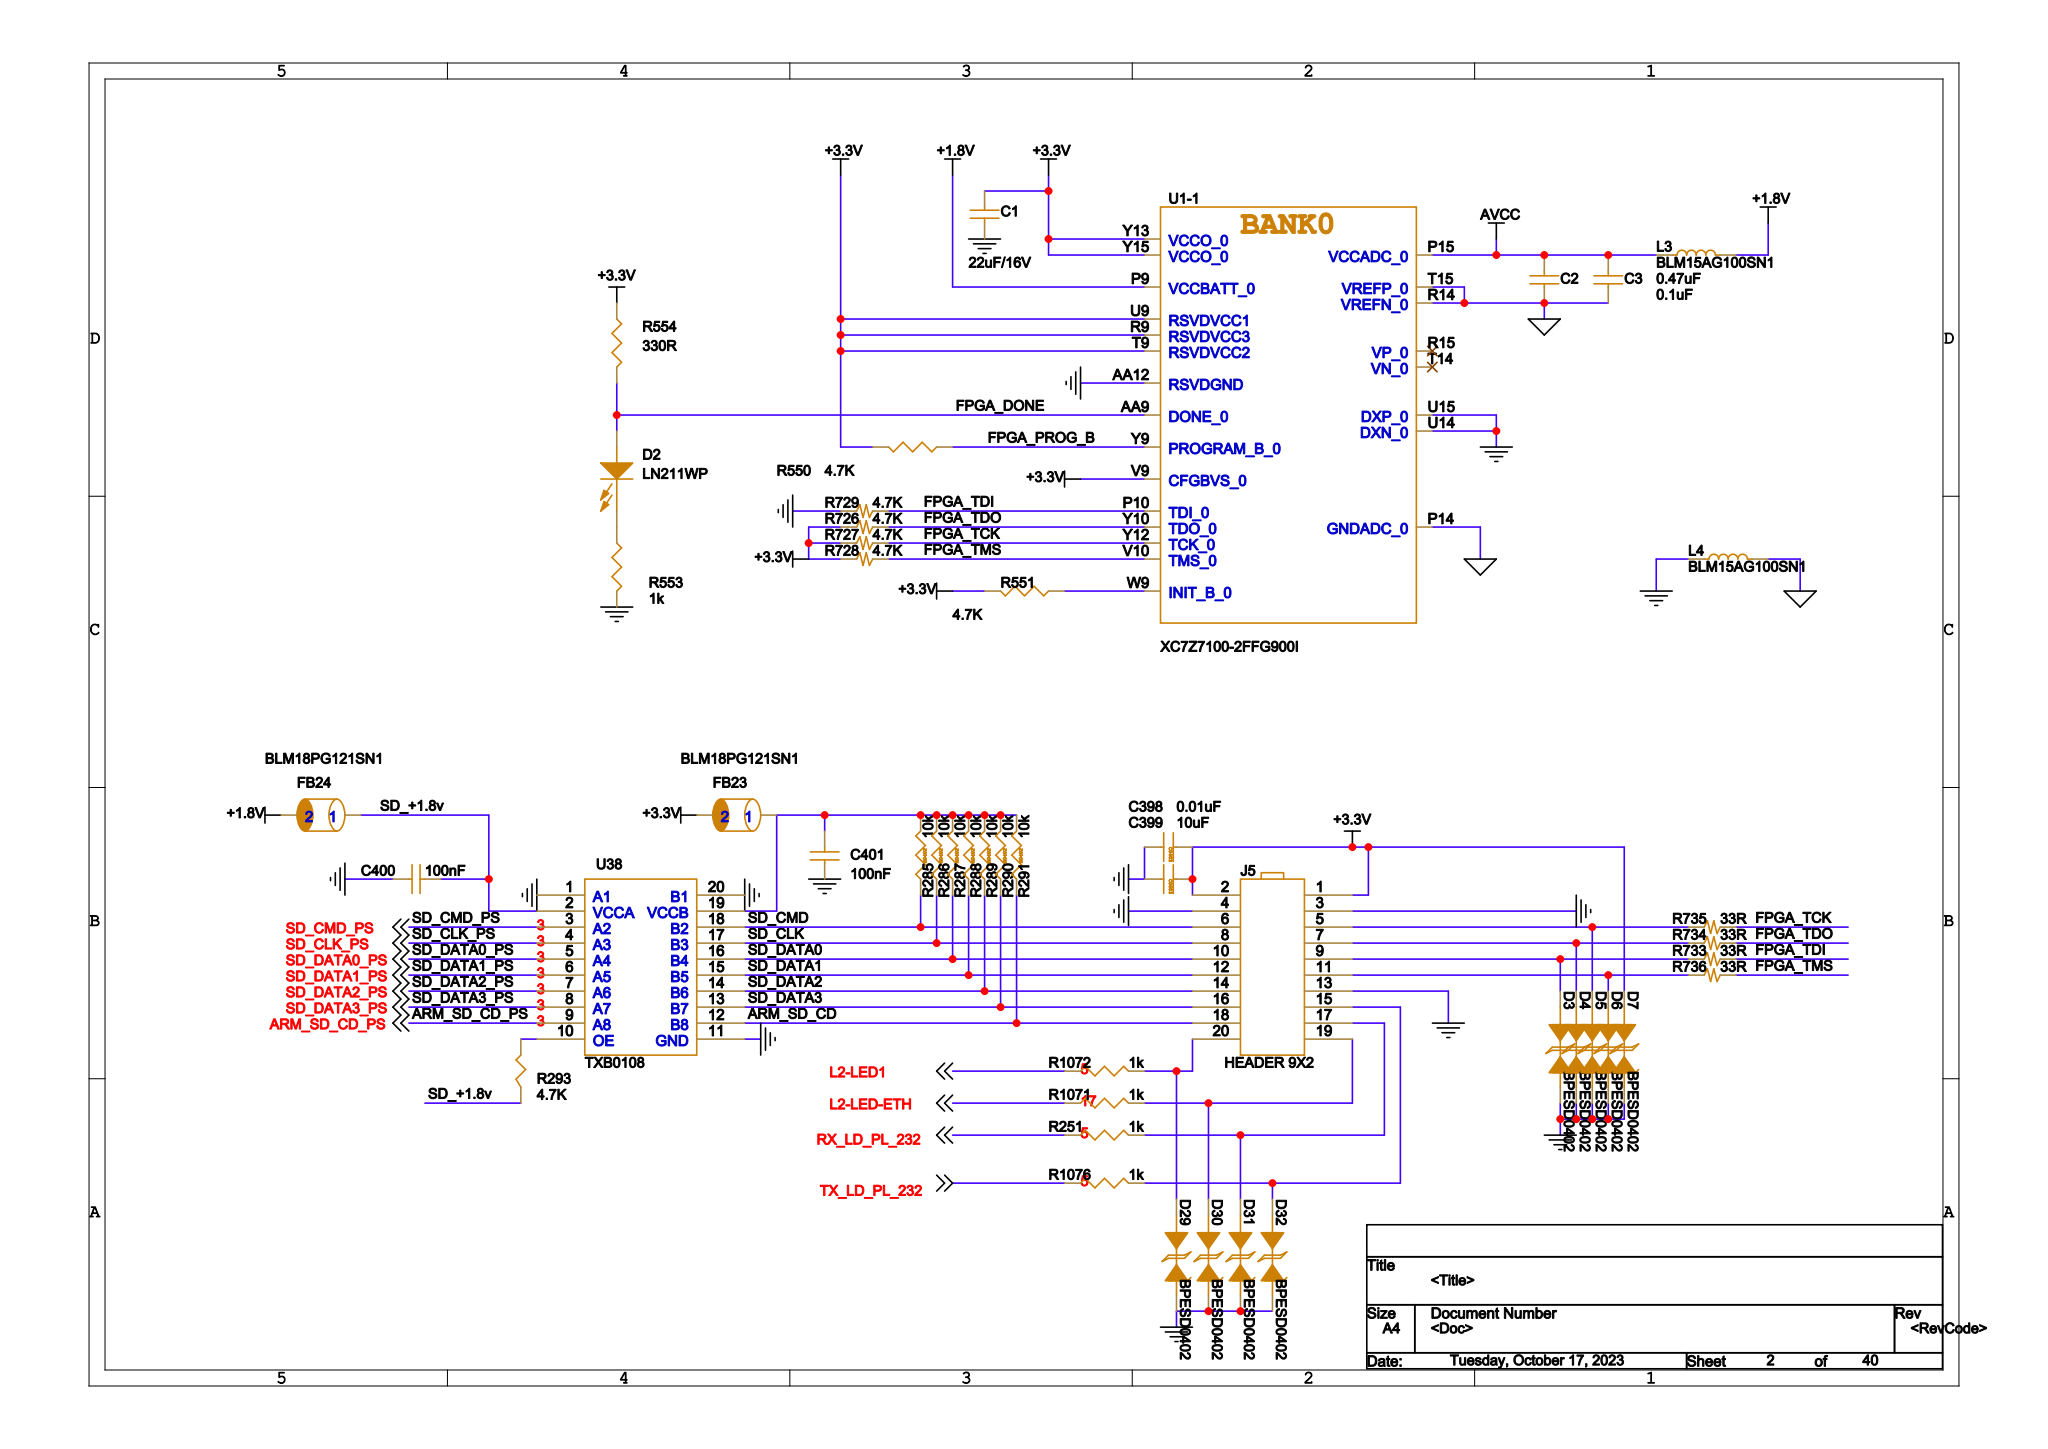Circuit board | Cadence Allegro | 1793 parts | 1223 nets | one sheet of the schematic
Parts on this sheet (reference | value | footprint):
C1 | 22uF/16V | C0603
C2 | 0.47uF | C0402
C3 | 0.1uF | C0402
C398 | 0.01uF | C0402
C399 | 10uF | C0402
C400 | 100nF | C0402
C401 | 100nF | C0402
D2 | LN211WP | D0603
D3 | BPESD0402 | C0402
D4 | BPESD0402 | C0402
D5 | BPESD0402 | C0402
D6 | BPESD0402 | C0402
D7 | BPESD0402 | C0402
D29 | BPESD0402 | C0402
D30 | BPESD0402 | C0402
D31 | BPESD0402 | C0402
D32 | BPESD0402 | C0402
FB23 | BLM18PG121SN1 | FB0603
FB24 | BLM18PG121SN1 | FB0603
J5 | HEADER 9X2 | DIP2X10_A
L3 | BLM15AG100SN1 | L0402
R251 | 1k | R0402
R285 | 10k | R0402
R286 | 10k | R0402
R287 | 10k | R0402
R288 | 10k | R0402
R289 | 10k | R0402
R290 | 10k | R0402
R291 | 10k | R0402
R293 | 4.7K | R0402
R550 | 4.7K | R0402
R551 | 4.7K | R0402
R553 | 1K | R0402
R554 | 330R | R0402
R726 | 4.7K | R0402
R727 | 4.7K | R0402
R728 | 4.7K | R0402
R729 | 4.7K | R0402
R733 | 33R | R0402
R734 | 33R | R0402
R735 | 33R | R0402
R736 | 33R | R0402
R1071 | 1k | R0402
R1072 | 1k | R0402
R1076 | 1k | R0402
U38 | TXB0108 | LC-TSSOP-20
Nets of these parts (net: part-pin ...):
GND: C1-2 C398-2 C399-2 C400-1 C401-1 D3-2 D4-2 D5-2 D6-2 D7-2 D29-2 D30-2 D31-2 D32-2 J5-3 J5-4 J5-13 R553-1 R729-2 U38-1 U38-11 U38-20
N18327447: D29-1 J5-20 R1072-1
N18321175: D3-1 J5-9 R733-2
N18327442: D30-1 J5-19 R1071-1
N18325115: D31-1 J5-17 R251-1
N18325094: D32-1 J5-15 R1076-1
N18321158: D4-1 J5-7 R734-2
N18321141: D5-1 J5-5 R735-2
N18321184: D6-1 J5-11 R736-2
+3.3V: C1-1 C398-1 C399-1 D7-1 FB23-2 J5-1 J5-2 R550-1 R551-1 R554-2 R726-2 R727-2 R728-2
SD_DATA0: J5-10 R287-1 U38-16
SD_DATA1: J5-12 R288-1 U38-15
SD_DATA2: J5-14 R289-1 U38-14
SD_DATA3: J5-16 R290-1 U38-13
ARM_SD_CD: J5-18 R291-1 U38-12
SD_CMD: J5-6 R285-1 U38-18
SD_CLK: J5-8 R286-1 U38-17
+1.8V: FB24-2 L3-2
AGND: C2-1 C3-1
AVCC: C2-2 C3-2 L3-1
L2-LED-ETH: R1071-2
L2-LED1: R1072-2
TX_LD_PL_232: R1076-2
RX_LD_PL_232: R251-2
FPGA_PROG_B: R550-2
N00783: R551-2
FPGA_DONE: D2-1 R554-1
SD_CMD_PS: U38-3
SD_CLK_PS: U38-4
SD_DATA0_PS: U38-5
SD_DATA1_PS: U38-6
SD_DATA2_PS: U38-7
SD_DATA3_PS: U38-8
ARM_SD_CD_PS: U38-9
N18326072: R293-2 U38-10
SD_+1.8V: C400-2 FB24-1 R293-1 U38-2
N18320094: C401-2 FB23-1 R285-2 R286-2 R287-2 R288-2 R289-2 R290-2 R291-2 U38-19
N019391: D2-2 R553-2
FPGA_TDO: R726-1 R734-1
FPGA_TCK: R727-1 R735-1
FPGA_TMS: R728-1 R736-1
FPGA_TDI: R729-1 R733-1